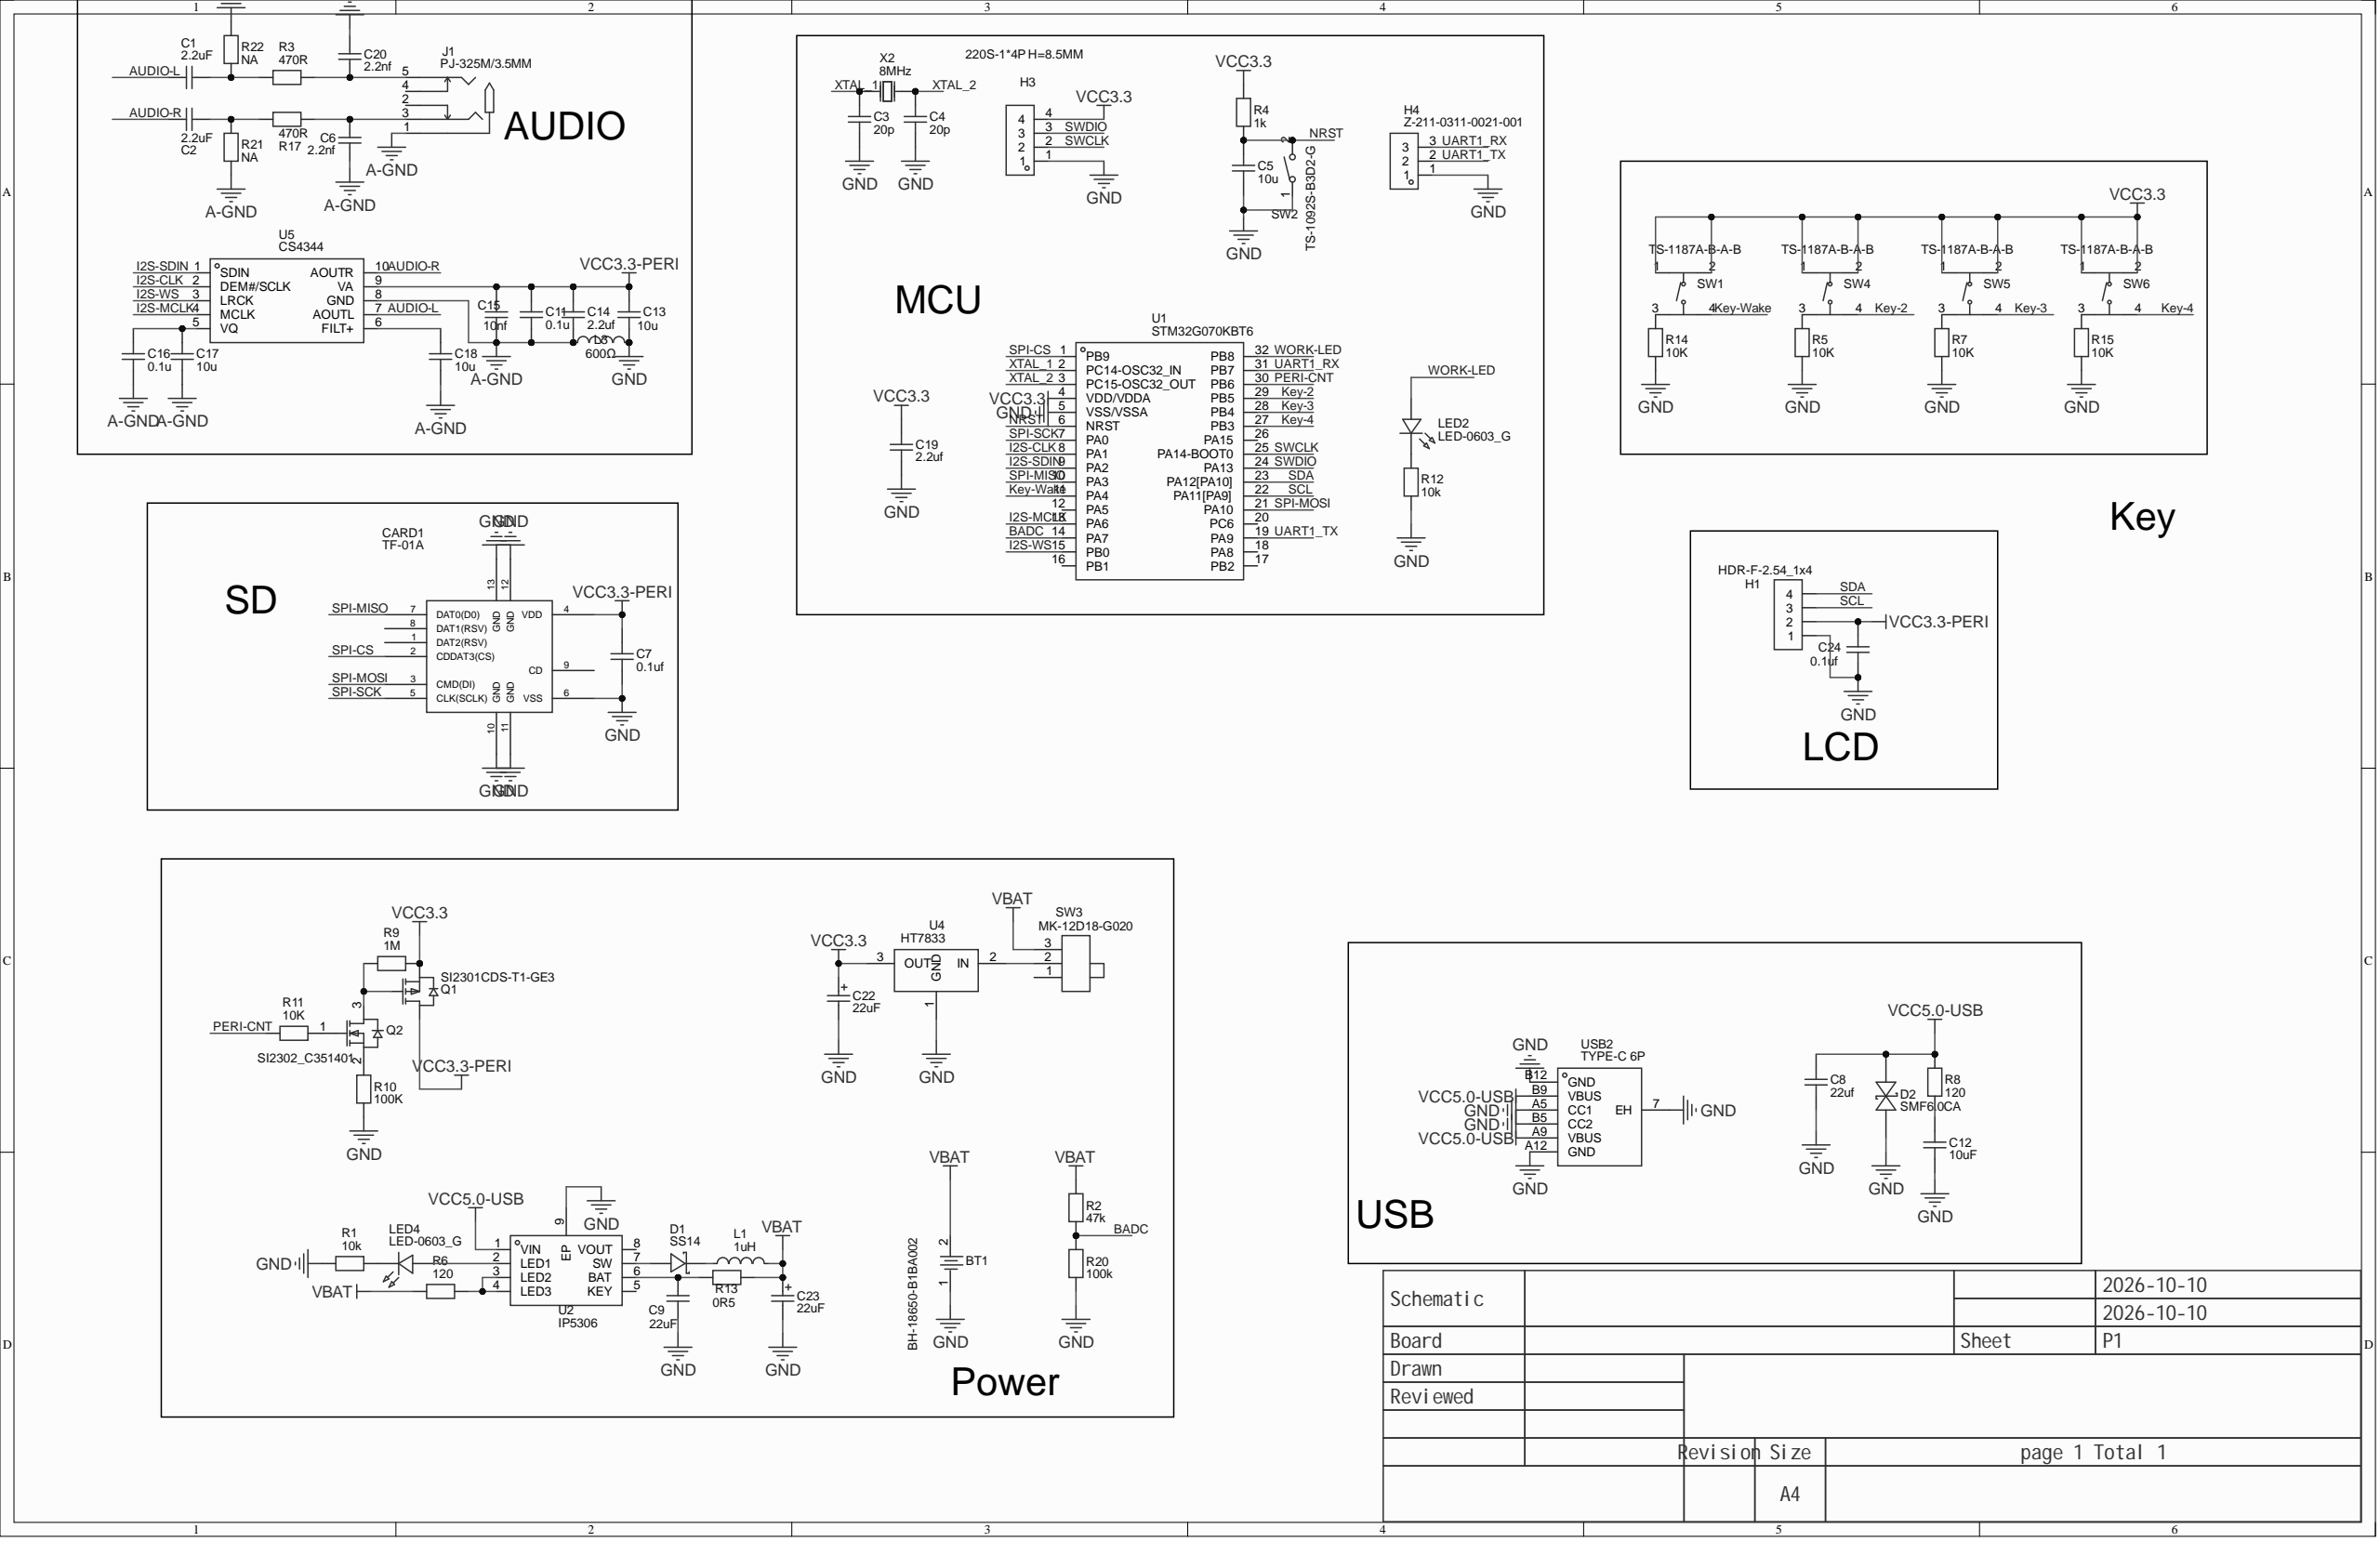Circuit board | Altium Designer | 67 parts | 54 nets
Bill of materials:
Comment,Description,Designator,Footprint,LibRef,Quantity
"BH-18650-B1BA002","","BT1","BATTERY-SMD_18650-1S-L77.1-W20.7-1","BH-18650-B1BA002","1"
"2.2uF","","C1, C2, C14, C19","C0603","CL10A225KO8NNNC, 2.2uf","4"
"20p","","C3, C4","C0603","20p","2"
"10u","","C5, C13, C17, C18","C0603","10u","4"
"2.2nf","","C6, C20","C0603","CL10A225KO8NNNC","2"
"0.1uf","","C7, C24","C0603","0.1uf","2"
"22uf","","C8, C9","C0603","0603X106M250NT, CC0603MRX5R5BB226","2"
"0.1u","","C11, C16","C0603","0.1u","2"
"10uF","","C12","C0603","0603X106M250NT","1"
"10nf","","C15","C0603","10nf","1"
"22uF","","C22, C23","CAP-SMD_L3.5-W2.8-R-RD","TAJB226K016RNJ","2"
"TF-01A","","CARD1","TF-SMD_TF-01A","TF-01A","1"
"SS14","","D1","SMA_L4.2-W2.6-LS5.3-RD","SS14","1"
"SMF6.0CA","","D2","SOD-123FL_L2.8-W1.8-LS3.7-BI","SMF6.0CA","1"
"HDR-F-2.54_1x4","","H1","HDR-F-2.54_1X4","HDR-F-2.54_1x4","1"
"220S-1*4P H=8.5MM","","H3","HDR-TH_4P-P2.54-V-F","220S-1*4P H=8.5MM Ytype Gold-plated","1"
"Z-211-0311-0021-001","","H4","HDR-TH_3P-P2.54-V-M-1","Z-211-0311-0021-001","1"
"PJ-325M/3.5MM","","J1","AUDIO-TH_PJ-325C","PJ-325M/3.5MM","1"
"1uH","","L1","IND-SMD_L6.8-W6.8_SMMS0630","SMMS0630-1R0M","1"
"600Ω","","L3","L1206","CBW321609U601T","1"
"LED-0603_G","","LED2, LED4","LED0603_GREEN","19-217/GHC-YR1S2/3T","2"
"SI2301CDS-T1-GE3","","Q1","SOT-23-3_L3.0-W1.7-P0.95-LS2.9-BR","SI2301CDS-T1-GE3","1"
"SI2302_C351401","","Q2","SOT-23-3_L2.9-W1.3-P1.90-LS2.4","SI2302","1"
"10k","","R1, R5, R7, R11, R12, R14, R15","R0603","10k","7"
"47k","","R2","R0603","47k","1"
"470R","","R3, R17","R0603","470R","2"
"1k","","R4","R0603","1k","1"
"120","","R6, R8","R0603","120","2"
"1M","","R9","R0603","1M","1"
"100K","","R10, R20","R0603","100K","2"
"0R5","","R13","R1206","1206W4F590LT5E","1"
"NA","","R21, R22","R0603","NA","2"
"TS-1187A-B-A-B","","SW1, SW4, SW5, SW6","SW-SMD_4P-L5.1-W5.1-P3.70-LS6.5-TL-2","TS-1187A-B-A-B","4"
"TS-1092S-B3D2-G","","SW2","SW-SMD_L6.1-W3.6-LS7.9","TS-1092S-B3D2-G","1"
"MK-12D18-G020","","SW3","SW-TH_MK-12D18-G040","MK-12D18-G020","1"
"STM32G070KBT6","","U1","LQFP-32_L7.0-W7.0-P0.80-LS9.0-BL","STM32G070KBT6","1"
"IP5306","","U2","ESOP-8_L4.9-W3.9-P1.27-LS6.0-BL-EP","IP5306","1"
"HT7833","","U4","SOT-89_L4.5-W2.5-P1.50-LS4.2-BR","HT7833","1"
"CS4344","","U5","TSSOP-10_L3.0-W3.0-P0.50-LS4.9-BL","CS4344","1"
"TYPE-C 6P","","USB2","TYPE-C-SMD_TYPE-C-6P","TYPE-C 6P","1"
"8MHz","","X2","CRYSTAL-SMD_L5.0-W3.2","X50328MSB2GI","1"
Netlist (Protel format):
[
BT1
BATTERY-SMD_18650-1S-L77.1-W20.7-1
BH-18650-B1BA002



]
[
C1
C0603
2.2uF



]
[
C2
C0603
2.2uF



]
[
C3
C0603
20p



]
[
C4
C0603
20p



]
[
C5
C0603
10u



]
[
C6
C0603
2.2nf



]
[
C7
C0603
0.1uf



]
[
C8
C0603
22uf



]
[
C9
C0603
22uF



]
[
C11
C0603
0.1u



]
[
C12
C0603
10uF



]
[
C13
C0603
10u



]
[
C14
C0603
2.2uf



]
[
C15
C0603
10nf



]
[
C16
C0603
0.1u



]
[
C17
C0603
10u



]
[
C18
C0603
10u



]
[
C19
C0603
2.2uf



]
[
C20
C0603
2.2nf



]
[
C22
CAP-SMD_L3.5-W2.8-R-RD
22uF



]
[
C23
CAP-SMD_L3.5-W2.8-R-RD
22uF



]
[
C24
C0603
0.1uf



]
[
CARD1
TF-SMD_TF-01A
TF-01A



]
[
D1
SMA_L4.2-W2.6-LS5.3-RD
SS14



]
[
D2
SOD-123FL_L2.8-W1.8-LS3.7-BI
SMF6.0CA



]
[
H1
HDR-F-2.54_1X4
HDR-F-2.54_1x4



]
[
H3
HDR-TH_4P-P2.54-V-F
220S-1*4P H=8.5MM



]
[
H4
HDR-TH_3P-P2.54-V-M-1
Z-211-0311-0021-001



]
[
J1
AUDIO-TH_PJ-325C
PJ-325M/3.5MM



]
[
L1
IND-SMD_L6.8-W6.8_SMMS0630
1uH



]
[
L3
L1206
600Ω



]
[
LED2
LED0603_GREEN
LED-0603_G



]
[
LED4
LED0603_GREEN
LED-0603_G



]
[
Q1
SOT-23-3_L3.0-W1.7-P0.95-LS2.9-BR
SI2301CDS-T1-GE3



]
[
Q2
SOT-23-3_L2.9-W1.3-P1.90-LS2.4
SI2302_C351401



]
[
R1
R0603
10k



]
[
R2
R0603
47k



]
[
R3
R0603
470R



]
[
R4
R0603
1k



]
[
R5
R0603
10K



]
[
R6
R0603
120



]
[
R7
R0603
10K



]
[
R8
R0603
120



]
[
R9
R0603
1M



]
[
R10
R0603
100K



]
[
R11
R0603
10K



]
[
R12
R0603
10k



]
[
R13
R1206
0R5



]
[
R14
R0603
10K



]
[
R15
R0603
10K



]
[
R17
R0603
470R



]
[
R20
R0603
100k



]
[
R21
R0603
NA



]
[
R22
R0603
NA



]
[
SW1
SW-SMD_4P-L5.1-W5.1-P3.70-LS6.5-TL-2
TS-1187A-B-A-B



]
[
SW2
SW-SMD_L6.1-W3.6-LS7.9
TS-1092S-B3D2-G



]
[
SW3
SW-TH_MK-12D18-G040
MK-12D18-G020



]
[
SW4
SW-SMD_4P-L5.1-W5.1-P3.70-LS6.5-TL-2
TS-1187A-B-A-B



]
[
SW5
SW-SMD_4P-L5.1-W5.1-P3.70-LS6.5-TL-2
TS-1187A-B-A-B



]
[
SW6
SW-SMD_4P-L5.1-W5.1-P3.70-LS6.5-TL-2
TS-1187A-B-A-B



]
[
U1
LQFP-32_L7.0-W7.0-P0.80-LS9.0-BL
STM32G070KBT6



]
[
U2
ESOP-8_L4.9-W3.9-P1.27-LS6.0-BL-EP
IP5306



]
[
U4
SOT-89_L4.5-W2.5-P1.50-LS4.2-BR
HT7833



]
[
U5
TSSOP-10_L3.0-W3.0-P0.50-LS4.9-BL
CS4344



]
[
USB2
TYPE-C-SMD_TYPE-C-6P
TYPE-C 6P



]
[
X2
CRYSTAL-SMD_L5.0-W3.2
8MHz



]
(
XTAL_2
C4-2
U1-3
X2-2
)
(
XTAL_1
C3-2
U1-2
X2-1
)
(
WORK-LED
LED2-1
U1-32
)
(
VCC5.0-USB
C8-2
D2-2
R8-1
U2-1
USB2-A9
USB2-B9
)
(
VCC3.3-PERI
C7-2
C11-2
C13-2
C14-2
C15-2
C24-2
CARD1-4
H1-2
Q1-3
U5-9
)
(
VCC3.3
C19-2
C22-1
H3-4
Q1-2
R4-2
R9-1
SW1-1
SW1-2
SW4-1
SW4-2
SW5-1
SW5-2
SW6-1
SW6-2
U1-4
U4-3
)
(
VBAT
BT1-2
C23-1
L1-2
R2-2
R6-2
R13-2
SW3-3
)
(
UART1_TX
H4-2
U1-19
)
(
UART1_RX
H4-3
U1-31
)
(
SWDIO
H3-3
U1-24
)
(
SWCLK
H3-2
U1-25
)
(
SPI-SCK
CARD1-5
U1-7
)
(
SPI-MOSI
CARD1-3
U1-21
)
(
SPI-MISO
CARD1-7
U1-10
)
(
SPI-CS
CARD1-2
U1-1
)
(
SDA
H1-4
U1-23
)
(
SCL
H1-3
U1-22
)
(
PERI-CNT
R11-1
U1-30
)
(
NRST
C5-2
R4-1
SW2-2
U1-6
)
(
NetSW3_2
SW3-2
U4-2
)
(
NetR15_2
R15-2
SW6-3
)
(
NetR14_2
R14-2
SW1-3
)
(
NetR7_2
R7-2
SW5-3
)
(
NetR6_1
R6-1
U2-3
U2-4
)
(
NetR5_2
R5-2
SW4-3
)
(
NetQ2_2
Q2-2
R10-1
)
(
NetQ2_1
Q2-1
R11-2
)
(
NetQ1_1
Q1-1
Q2-3
R9-2
)
(
NetLED4_2
LED4-2
R1-1
)
(
NetLED4_1
LED4-1
U2-2
)
(
NetLED2_2
LED2-2
R12-2
)
(
NetD1_2
D1-2
U2-7
)
(
NetD1_1
D1-1
L1-1
)
(
NetC20_1
C20-1
J1-5
R3-1
)
(
NetC18_2
C18-2
U5-6
)
(
NetC16_2
C16-2
C17-2
U5-5
)
(
NetC12_2
C12-2
R8-2
)
(
NetC9_2
C9-2
R13-1
U2-6
)
(
NetC6_2
C6-2
J1-3
R17-1
)
(
NetC2_2
C2-2
R17-2
R21-1
)
(
NetC1_2
C1-2
R3-2
R22-2
)
(
Key-Wake
SW1-4
U1-11
)
(
Key-4
SW6-4
U1-27
)
(
Key-3
SW5-4
U1-28
)
(
Key-2
SW4-4
U1-29
)
(
I2S-WS
U1-15
U5-3
)
(
I2S-SDIN
U1-9
U5-1
)
(
I2S-MCLK
U1-13
U5-4
)
(
I2S-CLK
U1-8
U5-2
)
(
GND
BT1-1
C3-1
C4-1
C5-1
C7-1
C8-1
C9-1
C12-1
C13-1
C19-1
C22-2
C23-2
C24-1
CARD1-6
CARD1-10
CARD1-11
CARD1-12
CARD1-13
D2-1
H1-1
H3-1
H4-1
L3-2
R1-2
R5-1
R7-1
R10-2
R12-1
R14-1
R15-1
R20-1
SW2-1
U1-5
U2-9
U4-1
USB2-7
USB2-A5
USB2-A12
USB2-B5
USB2-B12
)
(
BADC
R2-1
R20-2
U1-14
)
(
AUDIO-R
C2-1
U5-10
)
(
AUDIO-L
C1-1
U5-7
)
(
A-GND
C6-1
C11-1
C14-1
C15-1
C16-1
C17-1
C18-1
C20-2
J1-1
L3-1
R21-2
R22-1
U5-8
)